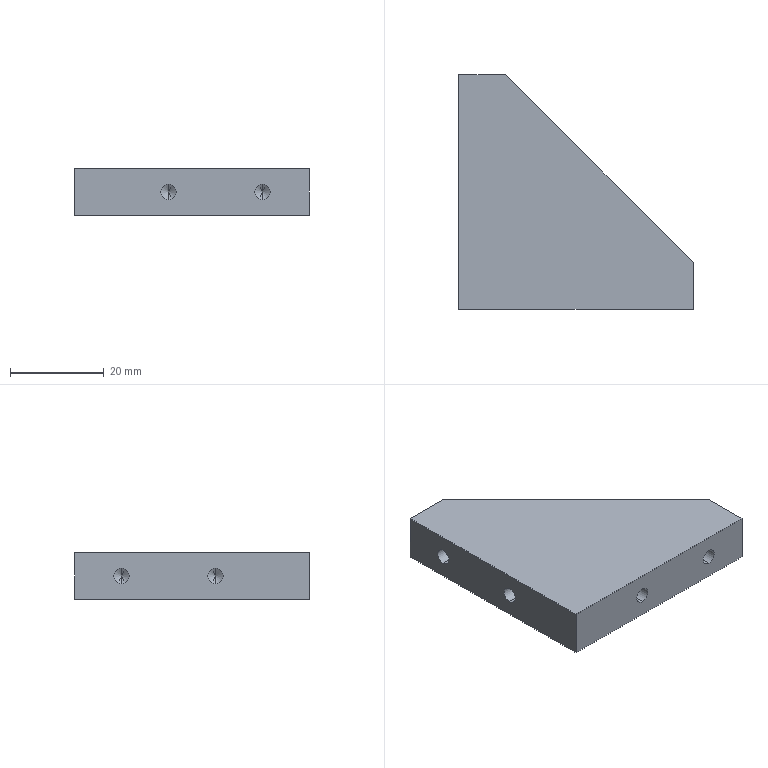Part | STEP file | 2084 Bag feed suction plate reinforcement | 1 solid | 23 faces | box 50 x 50 x 10 mm | volume 16595 mm3 | cylinder 8 | cone 8 | plane 7 | commonest cylinder face diameters 3.3 x8